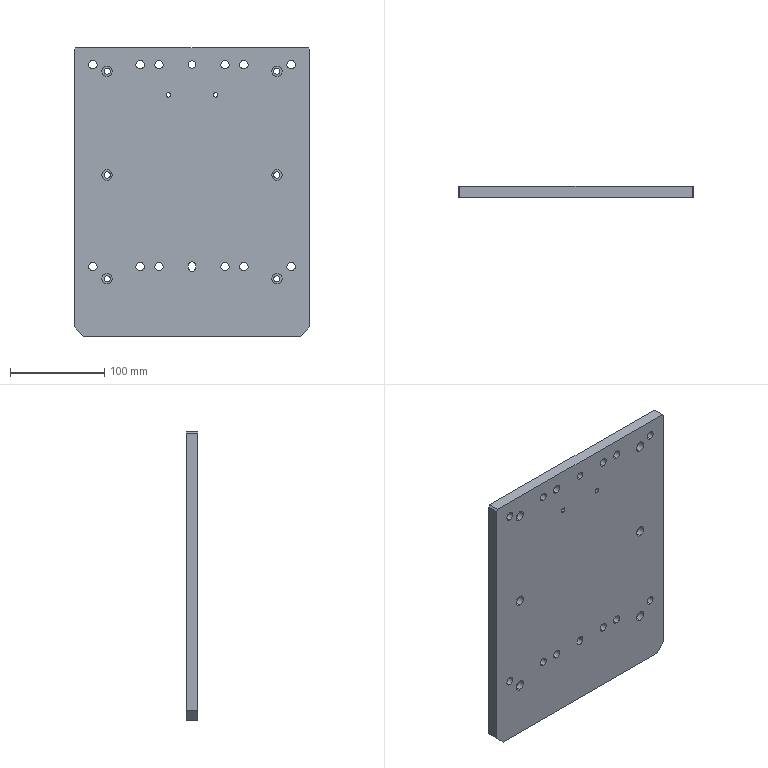Part | SolidWorks | features HoleWzd 5, Chamfer 2, Extrusion 1, ICE 1 | 1 solid | 87 faces | box 250 x 12 x 306 mm | volume 899864 mm3 | cylinder 63 | plane 18 | cone 6 | commonest cylinder face diameters 9 x24 6.6 x12 11 x12 5 x10 8 x5